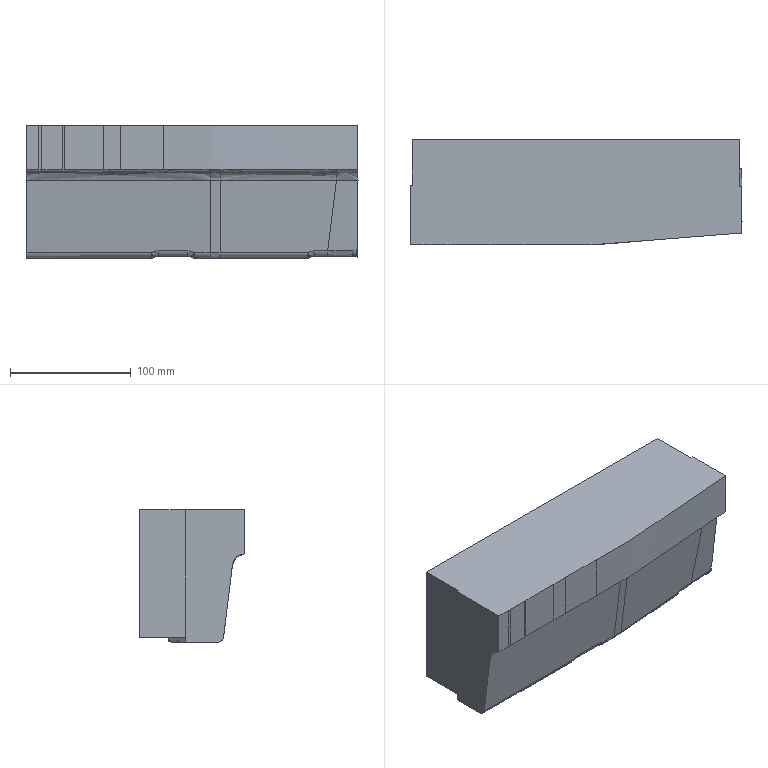Part | NX | features solid 2 | 1 solid | 94 faces | box 275.042 x 86.994 x 109.55 mm | volume 2236221 mm3 | spline 80 | plane 14